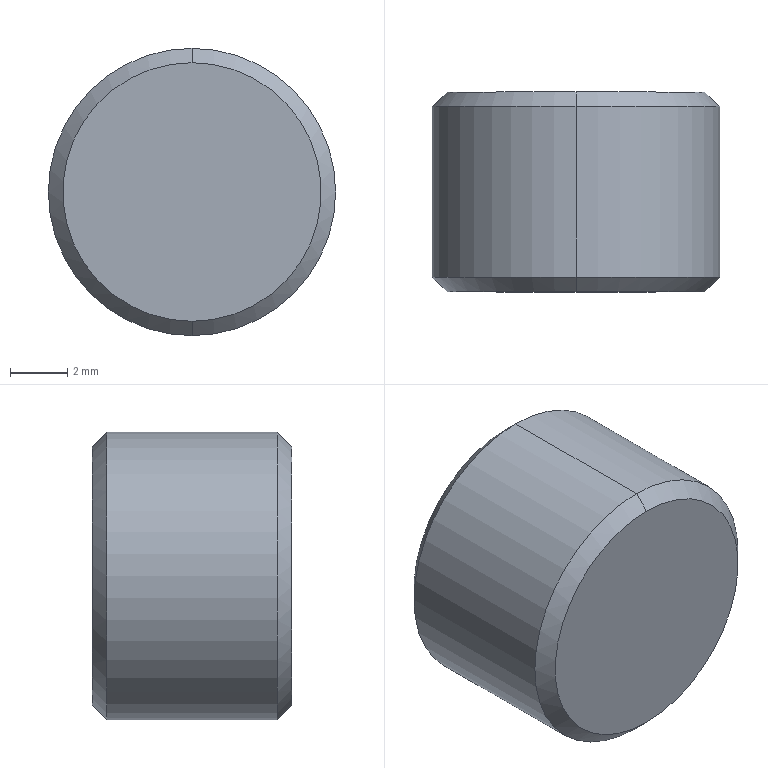Part | STEP file | 982 plug (1-8 plug) | 1 solid | 17 faces | box 10 x 6.95 x 10 mm | volume 421.396 mm3 | plane 9 | cone 6 | cylinder 2 | commonest cylinder face diameters 10 x2